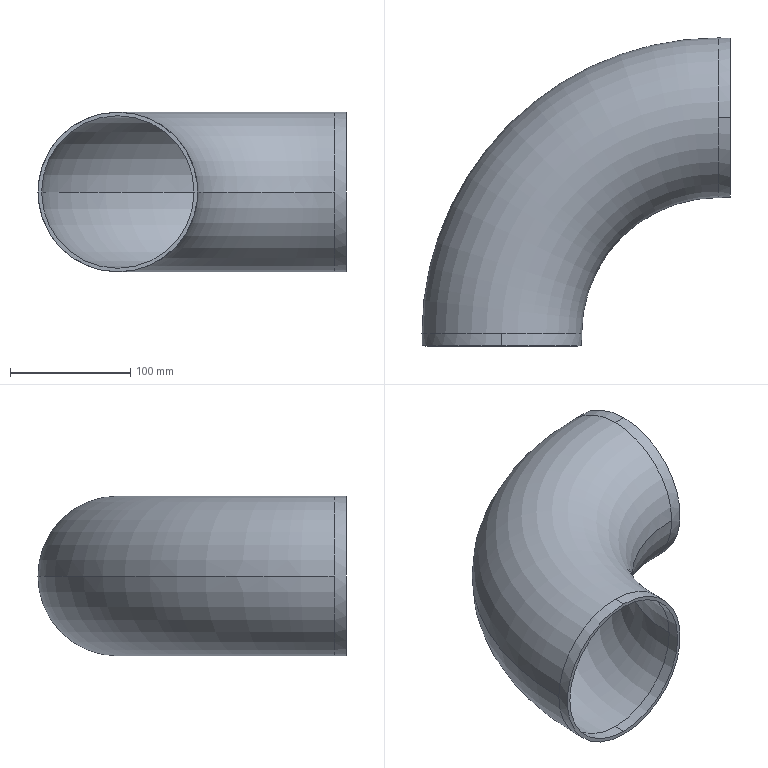Part | SolidWorks | features 3DProfileFeature 1, Shell 1, Sweep 1 | 1 solid | 14 faces | box 256.5 x 256.5 x 133 mm | volume 370928 mm3 | cylinder 8 | torus 4 | plane 2 | commonest cylinder face diameters 127 x4 133 x4
STEP:
#1=CARTESIAN_POINT('',(-63.5,10.,0.));
#2=VERTEX_POINT('',#1);
#3=CARTESIAN_POINT('',(0.,10.,63.5));
#4=VERTEX_POINT('',#3);
#5=CARTESIAN_POINT('',(0.,10.,0.));
#6=DIRECTION('',(0.,1.,0.));
#7=DIRECTION('',(0.,0.,-1.));
#8=AXIS2_PLACEMENT_3D('',#5,#6,#7);
#9=CIRCLE('',#8,63.5);
#10=EDGE_CURVE('',#2,#4,#9,.T.);
#11=ORIENTED_EDGE('',*,*,#10,.F.);
#12=CARTESIAN_POINT('',(180.,253.5,0.));
#13=VERTEX_POINT('',#12);
#14=CARTESIAN_POINT('',(180.,10.,0.));
#15=DIRECTION('',(0.,0.,-1.));
#16=DIRECTION('',(-1.,0.,0.));
#17=AXIS2_PLACEMENT_3D('',#14,#15,#16);
#18=CIRCLE('',#17,243.5);
#19=EDGE_CURVE('',#2,#13,#18,.T.);
#20=ORIENTED_EDGE('',*,*,#19,.T.);
#21=CARTESIAN_POINT('',(180.,190.,63.5));
#22=VERTEX_POINT('',#21);
#23=CARTESIAN_POINT('',(180.,190.,0.));
#24=DIRECTION('',(1.,0.,0.));
#25=DIRECTION('',(0.,0.,-1.));
#26=AXIS2_PLACEMENT_3D('',#23,#24,#25);
#27=CIRCLE('',#26,63.5);
#28=EDGE_CURVE('',#13,#22,#27,.T.);
#29=ORIENTED_EDGE('',*,*,#28,.T.);
#30=CARTESIAN_POINT('',(180.,126.5,0.));
#31=VERTEX_POINT('',#30);
#32=CARTESIAN_POINT('',(180.,190.,0.));
#33=DIRECTION('',(1.,0.,0.));
#34=DIRECTION('',(0.,0.,-1.));
#35=AXIS2_PLACEMENT_3D('',#32,#33,#34);
#36=CIRCLE('',#35,63.5);
#37=EDGE_CURVE('',#22,#31,#36,.T.);
#38=ORIENTED_EDGE('',*,*,#37,.T.);
#39=CARTESIAN_POINT('',(63.5,10.,0.));
#40=VERTEX_POINT('',#39);
#41=CARTESIAN_POINT('',(180.,10.,0.));
#42=DIRECTION('',(0.,0.,-1.));
#43=DIRECTION('',(-1.,0.,0.));
#44=AXIS2_PLACEMENT_3D('',#41,#42,#43);
#45=CIRCLE('',#44,116.5);
#46=EDGE_CURVE('',#40,#31,#45,.T.);
#47=ORIENTED_EDGE('',*,*,#46,.F.);
#48=CARTESIAN_POINT('',(0.,10.,0.));
#49=DIRECTION('',(0.,1.,0.));
#50=DIRECTION('',(0.,0.,-1.));
#51=AXIS2_PLACEMENT_3D('',#48,#49,#50);
#52=CIRCLE('',#51,63.5);
#53=EDGE_CURVE('',#4,#40,#52,.T.);
#54=ORIENTED_EDGE('',*,*,#53,.F.);
#55=EDGE_LOOP('',(#11,#20,#29,#38,#47,#54));
#56=FACE_OUTER_BOUND('',#55,.T.);
#57=CARTESIAN_POINT('',(180.,10.,0.));
#58=DIRECTION('',(0.,0.,-1.));
#59=DIRECTION('',(-1.,0.,0.));
#60=AXIS2_PLACEMENT_3D('',#57,#58,#59);
#61=TOROIDAL_SURFACE('',#60,180.,63.5);
#62=ADVANCED_FACE('',(#56),#61,.F.);
#63=CARTESIAN_POINT('',(0.,10.,-66.5));
#64=VERTEX_POINT('',#63);
#65=CARTESIAN_POINT('',(-66.5,10.,0.));
#66=VERTEX_POINT('',#65);
#67=CARTESIAN_POINT('',(0.,10.,0.));
#68=DIRECTION('',(0.,1.,0.));
#69=DIRECTION('',(0.,0.,1.));
#70=AXIS2_PLACEMENT_3D('',#67,#68,#69);
#71=CIRCLE('',#70,66.5);
#72=EDGE_CURVE('',#64,#66,#71,.T.);
#73=ORIENTED_EDGE('',*,*,#72,.T.);
#74=CARTESIAN_POINT('',(180.,256.5,0.));
#75=VERTEX_POINT('',#74);
#76=CARTESIAN_POINT('',(180.,10.,0.));
#77=DIRECTION('',(0.,0.,-1.));
#78=DIRECTION('',(-1.,0.,0.));
#79=AXIS2_PLACEMENT_3D('',#76,#77,#78);
#80=CIRCLE('',#79,246.5);
#81=EDGE_CURVE('',#66,#75,#80,.T.);
#82=ORIENTED_EDGE('',*,*,#81,.T.);
#83=CARTESIAN_POINT('',(180.,190.,-66.5));
#84=VERTEX_POINT('',#83);
#85=CARTESIAN_POINT('',(180.,190.,0.));
#86=DIRECTION('',(1.,0.,0.));
#87=DIRECTION('',(0.,0.,1.));
#88=AXIS2_PLACEMENT_3D('',#85,#86,#87);
#89=CIRCLE('',#88,66.5);
#90=EDGE_CURVE('',#84,#75,#89,.T.);
#91=ORIENTED_EDGE('',*,*,#90,.F.);
#92=CARTESIAN_POINT('',(180.,123.5,0.));
#93=VERTEX_POINT('',#92);
#94=CARTESIAN_POINT('',(180.,190.,0.));
#95=DIRECTION('',(1.,0.,0.));
#96=DIRECTION('',(0.,0.,1.));
#97=AXIS2_PLACEMENT_3D('',#94,#95,#96);
#98=CIRCLE('',#97,66.5);
#99=EDGE_CURVE('',#93,#84,#98,.T.);
#100=ORIENTED_EDGE('',*,*,#99,.F.);
#101=CARTESIAN_POINT('',(66.5,10.,0.));
#102=VERTEX_POINT('',#101);
#103=CARTESIAN_POINT('',(180.,10.,0.));
#104=DIRECTION('',(0.,0.,-1.));
#105=DIRECTION('',(-1.,0.,0.));
#106=AXIS2_PLACEMENT_3D('',#103,#104,#105);
#107=CIRCLE('',#106,113.5);
#108=EDGE_CURVE('',#102,#93,#107,.T.);
#109=ORIENTED_EDGE('',*,*,#108,.F.);
#110=CARTESIAN_POINT('',(0.,10.,0.));
#111=DIRECTION('',(0.,1.,0.));
#112=DIRECTION('',(0.,0.,1.));
#113=AXIS2_PLACEMENT_3D('',#110,#111,#112);
#114=CIRCLE('',#113,66.5);
#115=EDGE_CURVE('',#102,#64,#114,.T.);
#116=ORIENTED_EDGE('',*,*,#115,.T.);
#117=EDGE_LOOP('',(#73,#82,#91,#100,#109,#116));
#118=FACE_OUTER_BOUND('',#117,.T.);
#119=CARTESIAN_POINT('',(180.,10.,0.));
#120=DIRECTION('',(0.,0.,-1.));
#121=DIRECTION('',(-1.,0.,0.));
#122=AXIS2_PLACEMENT_3D('',#119,#120,#121);
#123=TOROIDAL_SURFACE('',#122,180.,66.5);
#124=ADVANCED_FACE('',(#118),#123,.T.);
#125=ORIENTED_EDGE('',*,*,#37,.F.);
#126=CARTESIAN_POINT('',(190.,190.,63.5));
#127=VERTEX_POINT('',#126);
#128=CARTESIAN_POINT('',(180.,190.,63.5));
#129=DIRECTION('',(1.,0.,0.));
#130=VECTOR('',#129,1000.);
#131=LINE('',#128,#130);
#132=EDGE_CURVE('',#22,#127,#131,.T.);
#133=ORIENTED_EDGE('',*,*,#132,.T.);
#134=CARTESIAN_POINT('',(190.,190.,-63.5));
#135=VERTEX_POINT('',#134);
#136=CARTESIAN_POINT('',(190.,190.,0.));
#137=DIRECTION('',(1.,0.,0.));
#138=DIRECTION('',(0.,0.,-1.));
#139=AXIS2_PLACEMENT_3D('',#136,#137,#138);
#140=CIRCLE('',#139,63.5);
#141=EDGE_CURVE('',#127,#135,#140,.T.);
#142=ORIENTED_EDGE('',*,*,#141,.T.);
#143=CARTESIAN_POINT('',(180.,190.,-63.5));
#144=VERTEX_POINT('',#143);
#145=CARTESIAN_POINT('',(180.,190.,-63.5));
#146=DIRECTION('',(1.,0.,0.));
#147=VECTOR('',#146,1000.);
#148=LINE('',#145,#147);
#149=EDGE_CURVE('',#144,#135,#148,.T.);
#150=ORIENTED_EDGE('',*,*,#149,.F.);
#151=CARTESIAN_POINT('',(180.,190.,0.));
#152=DIRECTION('',(1.,0.,0.));
#153=DIRECTION('',(0.,0.,-1.));
#154=AXIS2_PLACEMENT_3D('',#151,#152,#153);
#155=CIRCLE('',#154,63.5);
#156=EDGE_CURVE('',#31,#144,#155,.T.);
#157=ORIENTED_EDGE('',*,*,#156,.F.);
#158=EDGE_LOOP('',(#125,#133,#142,#150,#157));
#159=FACE_OUTER_BOUND('',#158,.T.);
#160=CARTESIAN_POINT('',(180.,190.,0.));
#161=DIRECTION('',(1.,0.,0.));
#162=DIRECTION('',(0.,0.,-1.));
#163=AXIS2_PLACEMENT_3D('',#160,#161,#162);
#164=CYLINDRICAL_SURFACE('',#163,63.5);
#165=ADVANCED_FACE('',(#159),#164,.F.);
#166=CARTESIAN_POINT('',(0.,0.,-63.5));
#167=VERTEX_POINT('',#166);
#168=CARTESIAN_POINT('',(0.,0.,63.5));
#169=VERTEX_POINT('',#168);
#170=CARTESIAN_POINT('',(0.,0.,0.));
#171=DIRECTION('',(0.,1.,0.));
#172=DIRECTION('',(0.,0.,1.));
#173=AXIS2_PLACEMENT_3D('',#170,#171,#172);
#174=CIRCLE('',#173,63.5);
#175=EDGE_CURVE('',#167,#169,#174,.T.);
#176=ORIENTED_EDGE('',*,*,#175,.F.);
#177=CARTESIAN_POINT('',(0.,10.,-63.5));
#178=VERTEX_POINT('',#177);
#179=CARTESIAN_POINT('',(0.,0.,-63.5));
#180=DIRECTION('',(0.,1.,0.));
#181=VECTOR('',#180,1000.);
#182=LINE('',#179,#181);
#183=EDGE_CURVE('',#167,#178,#182,.T.);
#184=ORIENTED_EDGE('',*,*,#183,.T.);
#185=CARTESIAN_POINT('',(0.,10.,0.));
#186=DIRECTION('',(0.,1.,0.));
#187=DIRECTION('',(0.,0.,-1.));
#188=AXIS2_PLACEMENT_3D('',#185,#186,#187);
#189=CIRCLE('',#188,63.5);
#190=EDGE_CURVE('',#178,#2,#189,.T.);
#191=ORIENTED_EDGE('',*,*,#190,.T.);
#192=ORIENTED_EDGE('',*,*,#10,.T.);
#193=CARTESIAN_POINT('',(0.,0.,63.5));
#194=DIRECTION('',(0.,1.,0.));
#195=VECTOR('',#194,1000.);
#196=LINE('',#193,#195);
#197=EDGE_CURVE('',#169,#4,#196,.T.);
#198=ORIENTED_EDGE('',*,*,#197,.F.);
#199=EDGE_LOOP('',(#176,#184,#191,#192,#198));
#200=FACE_OUTER_BOUND('',#199,.T.);
#201=CARTESIAN_POINT('',(0.,0.,0.));
#202=DIRECTION('',(0.,1.,0.));
#203=DIRECTION('',(0.,0.,1.));
#204=AXIS2_PLACEMENT_3D('',#201,#202,#203);
#205=CYLINDRICAL_SURFACE('',#204,63.5);
#206=ADVANCED_FACE('',(#200),#205,.F.);
#207=ORIENTED_EDGE('',*,*,#90,.T.);
#208=CARTESIAN_POINT('',(180.,190.,66.5));
#209=VERTEX_POINT('',#208);
#210=CARTESIAN_POINT('',(180.,190.,0.));
#211=DIRECTION('',(1.,0.,0.));
#212=DIRECTION('',(0.,0.,1.));
#213=AXIS2_PLACEMENT_3D('',#210,#211,#212);
#214=CIRCLE('',#213,66.5);
#215=EDGE_CURVE('',#75,#209,#214,.T.);
#216=ORIENTED_EDGE('',*,*,#215,.T.);
#217=CARTESIAN_POINT('',(190.,190.,66.5));
#218=VERTEX_POINT('',#217);
#219=CARTESIAN_POINT('',(180.,190.,66.5));
#220=DIRECTION('',(1.,0.,0.));
#221=VECTOR('',#220,1000.);
#222=LINE('',#219,#221);
#223=EDGE_CURVE('',#209,#218,#222,.T.);
#224=ORIENTED_EDGE('',*,*,#223,.T.);
#225=CARTESIAN_POINT('',(190.,190.,-66.5));
#226=VERTEX_POINT('',#225);
#227=CARTESIAN_POINT('',(190.,190.,0.));
#228=DIRECTION('',(1.,0.,0.));
#229=DIRECTION('',(0.,0.,1.));
#230=AXIS2_PLACEMENT_3D('',#227,#228,#229);
#231=CIRCLE('',#230,66.5);
#232=EDGE_CURVE('',#226,#218,#231,.T.);
#233=ORIENTED_EDGE('',*,*,#232,.F.);
#234=CARTESIAN_POINT('',(180.,190.,-66.5));
#235=DIRECTION('',(1.,0.,0.));
#236=VECTOR('',#235,1000.);
#237=LINE('',#234,#236);
#238=EDGE_CURVE('',#84,#226,#237,.T.);
#239=ORIENTED_EDGE('',*,*,#238,.F.);
#240=EDGE_LOOP('',(#207,#216,#224,#233,#239));
#241=FACE_OUTER_BOUND('',#240,.T.);
#242=CARTESIAN_POINT('',(180.,190.,0.));
#243=DIRECTION('',(1.,0.,0.));
#244=DIRECTION('',(0.,0.,-1.));
#245=AXIS2_PLACEMENT_3D('',#242,#243,#244);
#246=CYLINDRICAL_SURFACE('',#245,66.5);
#247=ADVANCED_FACE('',(#241),#246,.T.);
#248=CARTESIAN_POINT('',(0.,0.,66.5));
#249=VERTEX_POINT('',#248);
#250=CARTESIAN_POINT('',(0.,0.,-66.5));
#251=VERTEX_POINT('',#250);
#252=CARTESIAN_POINT('',(0.,0.,0.));
#253=DIRECTION('',(0.,1.,0.));
#254=DIRECTION('',(0.,0.,1.));
#255=AXIS2_PLACEMENT_3D('',#252,#253,#254);
#256=CIRCLE('',#255,66.5);
#257=EDGE_CURVE('',#249,#251,#256,.T.);
#258=ORIENTED_EDGE('',*,*,#257,.T.);
#259=CARTESIAN_POINT('',(0.,0.,-66.5));
#260=DIRECTION('',(0.,1.,0.));
#261=VECTOR('',#260,1000.);
#262=LINE('',#259,#261);
#263=EDGE_CURVE('',#251,#64,#262,.T.);
#264=ORIENTED_EDGE('',*,*,#263,.T.);
#265=ORIENTED_EDGE('',*,*,#115,.F.);
#266=CARTESIAN_POINT('',(0.,10.,66.5));
#267=VERTEX_POINT('',#266);
#268=CARTESIAN_POINT('',(0.,10.,0.));
#269=DIRECTION('',(0.,1.,0.));
#270=DIRECTION('',(0.,0.,1.));
#271=AXIS2_PLACEMENT_3D('',#268,#269,#270);
#272=CIRCLE('',#271,66.5);
#273=EDGE_CURVE('',#267,#102,#272,.T.);
#274=ORIENTED_EDGE('',*,*,#273,.F.);
#275=CARTESIAN_POINT('',(0.,0.,66.5));
#276=DIRECTION('',(0.,1.,0.));
#277=VECTOR('',#276,1000.);
#278=LINE('',#275,#277);
#279=EDGE_CURVE('',#249,#267,#278,.T.);
#280=ORIENTED_EDGE('',*,*,#279,.F.);
#281=EDGE_LOOP('',(#258,#264,#265,#274,#280));
#282=FACE_OUTER_BOUND('',#281,.T.);
#283=CARTESIAN_POINT('',(0.,0.,0.));
#284=DIRECTION('',(0.,1.,0.));
#285=DIRECTION('',(0.,0.,1.));
#286=AXIS2_PLACEMENT_3D('',#283,#284,#285);
#287=CYLINDRICAL_SURFACE('',#286,66.5);
#288=ADVANCED_FACE('',(#282),#287,.T.);
#289=ORIENTED_EDGE('',*,*,#223,.F.);
#290=CARTESIAN_POINT('',(180.,190.,0.));
#291=DIRECTION('',(1.,0.,0.));
#292=DIRECTION('',(0.,0.,1.));
#293=AXIS2_PLACEMENT_3D('',#290,#291,#292);
#294=CIRCLE('',#293,66.5);
#295=EDGE_CURVE('',#209,#93,#294,.T.);
#296=ORIENTED_EDGE('',*,*,#295,.T.);
#297=ORIENTED_EDGE('',*,*,#99,.T.);
#298=ORIENTED_EDGE('',*,*,#238,.T.);
#299=CARTESIAN_POINT('',(190.,190.,0.));
#300=DIRECTION('',(1.,0.,0.));
#301=DIRECTION('',(0.,0.,1.));
#302=AXIS2_PLACEMENT_3D('',#299,#300,#301);
#303=CIRCLE('',#302,66.5);
#304=EDGE_CURVE('',#218,#226,#303,.T.);
#305=ORIENTED_EDGE('',*,*,#304,.F.);
#306=EDGE_LOOP('',(#289,#296,#297,#298,#305));
#307=FACE_OUTER_BOUND('',#306,.T.);
#308=CARTESIAN_POINT('',(180.,190.,0.));
#309=DIRECTION('',(1.,0.,0.));
#310=DIRECTION('',(0.,0.,-1.));
#311=AXIS2_PLACEMENT_3D('',#308,#309,#310);
#312=CYLINDRICAL_SURFACE('',#311,66.5);
#313=ADVANCED_FACE('',(#307),#312,.T.);
#314=ORIENTED_EDGE('',*,*,#81,.F.);
#315=CARTESIAN_POINT('',(0.,10.,0.));
#316=DIRECTION('',(0.,1.,0.));
#317=DIRECTION('',(0.,0.,1.));
#318=AXIS2_PLACEMENT_3D('',#315,#316,#317);
#319=CIRCLE('',#318,66.5);
#320=EDGE_CURVE('',#66,#267,#319,.T.);
#321=ORIENTED_EDGE('',*,*,#320,.T.);
#322=ORIENTED_EDGE('',*,*,#273,.T.);
#323=ORIENTED_EDGE('',*,*,#108,.T.);
#324=ORIENTED_EDGE('',*,*,#295,.F.);
#325=ORIENTED_EDGE('',*,*,#215,.F.);
#326=EDGE_LOOP('',(#314,#321,#322,#323,#324,#325));
#327=FACE_OUTER_BOUND('',#326,.T.);
#328=CARTESIAN_POINT('',(180.,10.,0.));
#329=DIRECTION('',(0.,0.,-1.));
#330=DIRECTION('',(-1.,0.,0.));
#331=AXIS2_PLACEMENT_3D('',#328,#329,#330);
#332=TOROIDAL_SURFACE('',#331,180.,66.5);
#333=ADVANCED_FACE('',(#327),#332,.T.);
#334=ORIENTED_EDGE('',*,*,#263,.F.);
#335=CARTESIAN_POINT('',(0.,0.,0.));
#336=DIRECTION('',(0.,1.,0.));
#337=DIRECTION('',(0.,0.,1.));
#338=AXIS2_PLACEMENT_3D('',#335,#336,#337);
#339=CIRCLE('',#338,66.5);
#340=EDGE_CURVE('',#251,#249,#339,.T.);
#341=ORIENTED_EDGE('',*,*,#340,.T.);
#342=ORIENTED_EDGE('',*,*,#279,.T.);
#343=ORIENTED_EDGE('',*,*,#320,.F.);
#344=ORIENTED_EDGE('',*,*,#72,.F.);
#345=EDGE_LOOP('',(#334,#341,#342,#343,#344));
#346=FACE_OUTER_BOUND('',#345,.T.);
#347=CARTESIAN_POINT('',(0.,0.,0.));
#348=DIRECTION('',(0.,1.,0.));
#349=DIRECTION('',(0.,0.,1.));
#350=AXIS2_PLACEMENT_3D('',#347,#348,#349);
#351=CYLINDRICAL_SURFACE('',#350,66.5);
#352=ADVANCED_FACE('',(#346),#351,.T.);
#353=CARTESIAN_POINT('',(190.,190.,0.));
#354=DIRECTION('',(1.,0.,0.));
#355=DIRECTION('',(0.,0.,-1.));
#356=AXIS2_PLACEMENT_3D('',#353,#354,#355);
#357=CIRCLE('',#356,63.5);
#358=EDGE_CURVE('',#135,#127,#357,.T.);
#359=ORIENTED_EDGE('',*,*,#358,.F.);
#360=ORIENTED_EDGE('',*,*,#141,.F.);
#361=EDGE_LOOP('',(#359,#360));
#362=FACE_BOUND('',#361,.T.);
#363=ORIENTED_EDGE('',*,*,#232,.T.);
#364=ORIENTED_EDGE('',*,*,#304,.T.);
#365=EDGE_LOOP('',(#363,#364));
#366=FACE_OUTER_BOUND('',#365,.T.);
#367=CARTESIAN_POINT('',(190.,190.,0.));
#368=DIRECTION('',(1.,0.,0.));
#369=DIRECTION('',(0.,0.,1.));
#370=AXIS2_PLACEMENT_3D('',#367,#368,#369);
#371=PLANE('',#370);
#372=ADVANCED_FACE('',(#362,#366),#371,.T.);
#373=CARTESIAN_POINT('',(0.,0.,0.));
#374=DIRECTION('',(0.,1.,0.));
#375=DIRECTION('',(0.,0.,1.));
#376=AXIS2_PLACEMENT_3D('',#373,#374,#375);
#377=CIRCLE('',#376,63.5);
#378=EDGE_CURVE('',#169,#167,#377,.T.);
#379=ORIENTED_EDGE('',*,*,#378,.T.);
#380=ORIENTED_EDGE('',*,*,#175,.T.);
#381=EDGE_LOOP('',(#379,#380));
#382=FACE_BOUND('',#381,.T.);
#383=ORIENTED_EDGE('',*,*,#257,.F.);
#384=ORIENTED_EDGE('',*,*,#340,.F.);
#385=EDGE_LOOP('',(#383,#384));
#386=FACE_OUTER_BOUND('',#385,.T.);
#387=CARTESIAN_POINT('',(0.,0.,0.));
#388=DIRECTION('',(0.,1.,0.));
#389=DIRECTION('',(0.,0.,1.));
#390=AXIS2_PLACEMENT_3D('',#387,#388,#389);
#391=PLANE('',#390);
#392=ADVANCED_FACE('',(#382,#386),#391,.F.);
#393=ORIENTED_EDGE('',*,*,#132,.F.);
#394=ORIENTED_EDGE('',*,*,#28,.F.);
#395=CARTESIAN_POINT('',(180.,190.,0.));
#396=DIRECTION('',(1.,0.,0.));
#397=DIRECTION('',(0.,0.,-1.));
#398=AXIS2_PLACEMENT_3D('',#395,#396,#397);
#399=CIRCLE('',#398,63.5);
#400=EDGE_CURVE('',#144,#13,#399,.T.);
#401=ORIENTED_EDGE('',*,*,#400,.F.);
#402=ORIENTED_EDGE('',*,*,#149,.T.);
#403=ORIENTED_EDGE('',*,*,#358,.T.);
#404=EDGE_LOOP('',(#393,#394,#401,#402,#403));
#405=FACE_OUTER_BOUND('',#404,.T.);
#406=CARTESIAN_POINT('',(180.,190.,0.));
#407=DIRECTION('',(1.,0.,0.));
#408=DIRECTION('',(0.,0.,-1.));
#409=AXIS2_PLACEMENT_3D('',#406,#407,#408);
#410=CYLINDRICAL_SURFACE('',#409,63.5);
#411=ADVANCED_FACE('',(#405),#410,.F.);
#412=ORIENTED_EDGE('',*,*,#19,.F.);
#413=ORIENTED_EDGE('',*,*,#190,.F.);
#414=CARTESIAN_POINT('',(0.,10.,0.));
#415=DIRECTION('',(0.,1.,0.));
#416=DIRECTION('',(0.,0.,-1.));
#417=AXIS2_PLACEMENT_3D('',#414,#415,#416);
#418=CIRCLE('',#417,63.5);
#419=EDGE_CURVE('',#40,#178,#418,.T.);
#420=ORIENTED_EDGE('',*,*,#419,.F.);
#421=ORIENTED_EDGE('',*,*,#46,.T.);
#422=ORIENTED_EDGE('',*,*,#156,.T.);
#423=ORIENTED_EDGE('',*,*,#400,.T.);
#424=EDGE_LOOP('',(#412,#413,#420,#421,#422,#423));
#425=FACE_OUTER_BOUND('',#424,.T.);
#426=CARTESIAN_POINT('',(180.,10.,0.));
#427=DIRECTION('',(0.,0.,-1.));
#428=DIRECTION('',(-1.,0.,0.));
#429=AXIS2_PLACEMENT_3D('',#426,#427,#428);
#430=TOROIDAL_SURFACE('',#429,180.,63.5);
#431=ADVANCED_FACE('',(#425),#430,.F.);
#432=ORIENTED_EDGE('',*,*,#183,.F.);
#433=ORIENTED_EDGE('',*,*,#378,.F.);
#434=ORIENTED_EDGE('',*,*,#197,.T.);
#435=ORIENTED_EDGE('',*,*,#53,.T.);
#436=ORIENTED_EDGE('',*,*,#419,.T.);
#437=EDGE_LOOP('',(#432,#433,#434,#435,#436));
#438=FACE_OUTER_BOUND('',#437,.T.);
#439=CARTESIAN_POINT('',(0.,0.,0.));
#440=DIRECTION('',(0.,1.,0.));
#441=DIRECTION('',(0.,0.,1.));
#442=AXIS2_PLACEMENT_3D('',#439,#440,#441);
#443=CYLINDRICAL_SURFACE('',#442,63.5);
#444=ADVANCED_FACE('',(#438),#443,.F.);
#445=CLOSED_SHELL('',(#62,#124,#165,#206,#247,#288,#313,#333,#352,#372,#392,#411,#431,#444));
#446=MANIFOLD_SOLID_BREP('',#445);
#447=CARTESIAN_POINT('',(0.,0.,0.));
#448=DIRECTION('',(0.,0.,1.));
#449=DIRECTION('',(1.,0.,0.));
#450=AXIS2_PLACEMENT_3D('',#447,#448,#449);
#451=(LENGTH_UNIT()NAMED_UNIT(*)SI_UNIT(.MILLI.,.METRE.));
#452=UNCERTAINTY_MEASURE_WITH_UNIT(LENGTH_MEASURE(0.00001),#451,'','');
#453=(NAMED_UNIT(*)PLANE_ANGLE_UNIT()SI_UNIT($,.RADIAN.));
#454=(NAMED_UNIT(*)SI_UNIT($,.STERADIAN.)SOLID_ANGLE_UNIT());
#455=(GEOMETRIC_REPRESENTATION_CONTEXT(3)GLOBAL_UNCERTAINTY_ASSIGNED_CONTEXT((#452))GLOBAL_UNIT_ASSIGNED_CONTEXT((#451,#453,#454))REPRESENTATION_CONTEXT('',''));
#456=ADVANCED_BREP_SHAPE_REPRESENTATION('',(#446,#450),#455);